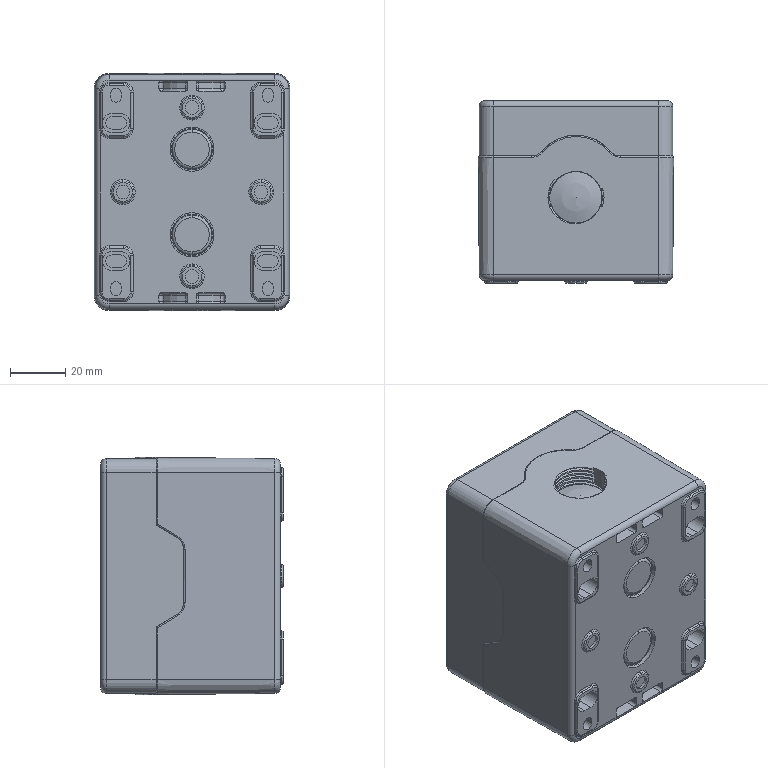Part | SolidWorks | features BaseBody 2 | 2 solids | 1986 faces | box 70.742 x 66 x 85.872 mm | volume 117624 mm3 | cylinder 788 | plane 766 | spline 211 | torus 156 | sphere 61 | cone 4 | commonest cylinder face diameters 7 x106 1 x105 6 x100 0.6 x72 7.6 x54 2 x48